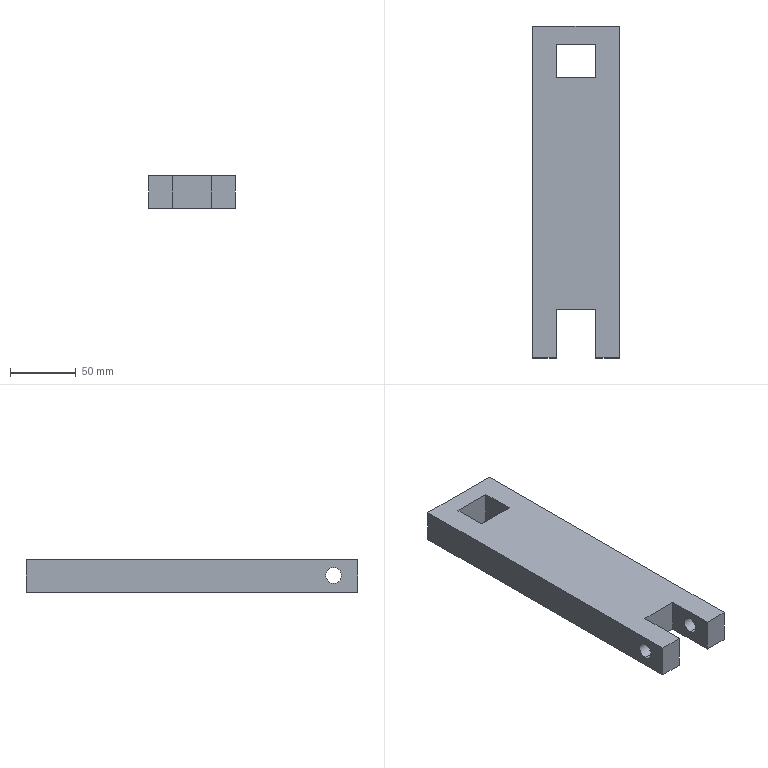Part | SolidWorks | features ICE 2, 3DProfileFeature 1, Extrusion 1, HoleWzd 1, MirrorPattern 1 | 1 solid | 18 faces | box 66 x 252 x 25 mm | volume 365157 mm3 | plane 14 | cylinder 4 | commonest cylinder face diameters 12 x4
STEP:
#1=CARTESIAN_POINT('',(-15.,-131.5,-5.548));
#2=VERTEX_POINT('',#1);
#3=CARTESIAN_POINT('',(-15.,-131.5,6.452));
#4=VERTEX_POINT('',#3);
#5=CARTESIAN_POINT('',(-15.,-131.5,0.4516));
#6=DIRECTION('',(-1.,0.,0.));
#7=DIRECTION('',(0.,0.,1.));
#8=AXIS2_PLACEMENT_3D('',#5,#6,#7);
#9=CIRCLE('',#8,6.);
#10=EDGE_CURVE('',#2,#4,#9,.T.);
#11=ORIENTED_EDGE('',*,*,#10,.F.);
#12=CARTESIAN_POINT('',(-33.,-131.5,-5.548));
#13=VERTEX_POINT('',#12);
#14=CARTESIAN_POINT('',(-33.,-131.5,-5.548));
#15=DIRECTION('',(-1.,0.,0.));
#16=VECTOR('',#15,1000.);
#17=LINE('',#14,#16);
#18=EDGE_CURVE('',#2,#13,#17,.T.);
#19=ORIENTED_EDGE('',*,*,#18,.T.);
#20=CARTESIAN_POINT('',(-33.,-131.5,6.452));
#21=VERTEX_POINT('',#20);
#22=CARTESIAN_POINT('',(-33.,-131.5,0.4516));
#23=DIRECTION('',(-1.,0.,0.));
#24=DIRECTION('',(0.,0.,1.));
#25=AXIS2_PLACEMENT_3D('',#22,#23,#24);
#26=CIRCLE('',#25,6.);
#27=EDGE_CURVE('',#13,#21,#26,.T.);
#28=ORIENTED_EDGE('',*,*,#27,.T.);
#29=CARTESIAN_POINT('',(-33.,-131.5,6.452));
#30=DIRECTION('',(-1.,0.,0.));
#31=VECTOR('',#30,1000.);
#32=LINE('',#29,#31);
#33=EDGE_CURVE('',#4,#21,#32,.T.);
#34=ORIENTED_EDGE('',*,*,#33,.F.);
#35=EDGE_LOOP('',(#11,#19,#28,#34));
#36=FACE_OUTER_BOUND('',#35,.T.);
#37=CARTESIAN_POINT('',(-33.,-131.5,0.4516));
#38=DIRECTION('',(-1.,0.,0.));
#39=DIRECTION('',(0.,0.,1.));
#40=AXIS2_PLACEMENT_3D('',#37,#38,#39);
#41=CYLINDRICAL_SURFACE('',#40,6.);
#42=ADVANCED_FACE('',(#36),#41,.F.);
#43=CARTESIAN_POINT('',(15.,-131.5,6.452));
#44=VERTEX_POINT('',#43);
#45=CARTESIAN_POINT('',(15.,-131.5,-5.548));
#46=VERTEX_POINT('',#45);
#47=CARTESIAN_POINT('',(15.,-131.5,0.4516));
#48=DIRECTION('',(1.,0.,0.));
#49=DIRECTION('',(0.,0.,-1.));
#50=AXIS2_PLACEMENT_3D('',#47,#48,#49);
#51=CIRCLE('',#50,6.);
#52=EDGE_CURVE('',#44,#46,#51,.T.);
#53=ORIENTED_EDGE('',*,*,#52,.F.);
#54=CARTESIAN_POINT('',(33.,-131.5,6.452));
#55=VERTEX_POINT('',#54);
#56=CARTESIAN_POINT('',(33.,-131.5,6.452));
#57=DIRECTION('',(1.,0.,0.));
#58=VECTOR('',#57,1000.);
#59=LINE('',#56,#58);
#60=EDGE_CURVE('',#44,#55,#59,.T.);
#61=ORIENTED_EDGE('',*,*,#60,.T.);
#62=CARTESIAN_POINT('',(33.,-131.5,-5.548));
#63=VERTEX_POINT('',#62);
#64=CARTESIAN_POINT('',(33.,-131.5,0.4516));
#65=DIRECTION('',(1.,0.,0.));
#66=DIRECTION('',(0.,0.,-1.));
#67=AXIS2_PLACEMENT_3D('',#64,#65,#66);
#68=CIRCLE('',#67,6.);
#69=EDGE_CURVE('',#55,#63,#68,.T.);
#70=ORIENTED_EDGE('',*,*,#69,.T.);
#71=CARTESIAN_POINT('',(33.,-131.5,-5.548));
#72=DIRECTION('',(1.,0.,0.));
#73=VECTOR('',#72,1000.);
#74=LINE('',#71,#73);
#75=EDGE_CURVE('',#46,#63,#74,.T.);
#76=ORIENTED_EDGE('',*,*,#75,.F.);
#77=EDGE_LOOP('',(#53,#61,#70,#76));
#78=FACE_OUTER_BOUND('',#77,.T.);
#79=CARTESIAN_POINT('',(33.,-131.5,0.4516));
#80=DIRECTION('',(1.,0.,0.));
#81=DIRECTION('',(0.,0.,-1.));
#82=AXIS2_PLACEMENT_3D('',#79,#80,#81);
#83=CYLINDRICAL_SURFACE('',#82,6.);
#84=ADVANCED_FACE('',(#78),#83,.F.);
#85=CARTESIAN_POINT('',(33.,-150.,-12.5));
#86=VERTEX_POINT('',#85);
#87=CARTESIAN_POINT('',(33.,102.,-12.5));
#88=VERTEX_POINT('',#87);
#89=CARTESIAN_POINT('',(33.,-150.,-12.5));
#90=DIRECTION('',(0.,1.,0.));
#91=VECTOR('',#90,1000.);
#92=LINE('',#89,#91);
#93=EDGE_CURVE('',#86,#88,#92,.T.);
#94=ORIENTED_EDGE('',*,*,#93,.T.);
#95=CARTESIAN_POINT('',(33.,102.,12.5));
#96=VERTEX_POINT('',#95);
#97=CARTESIAN_POINT('',(33.,102.,12.5));
#98=DIRECTION('',(0.,0.,-1.));
#99=VECTOR('',#98,1000.);
#100=LINE('',#97,#99);
#101=EDGE_CURVE('',#96,#88,#100,.T.);
#102=ORIENTED_EDGE('',*,*,#101,.F.);
#103=CARTESIAN_POINT('',(33.,-150.,12.5));
#104=VERTEX_POINT('',#103);
#105=CARTESIAN_POINT('',(33.,-150.,12.5));
#106=DIRECTION('',(0.,1.,0.));
#107=VECTOR('',#106,1000.);
#108=LINE('',#105,#107);
#109=EDGE_CURVE('',#104,#96,#108,.T.);
#110=ORIENTED_EDGE('',*,*,#109,.F.);
#111=CARTESIAN_POINT('',(33.,-150.,12.5));
#112=DIRECTION('',(0.,0.,-1.));
#113=VECTOR('',#112,1000.);
#114=LINE('',#111,#113);
#115=EDGE_CURVE('',#104,#86,#114,.T.);
#116=ORIENTED_EDGE('',*,*,#115,.T.);
#117=EDGE_LOOP('',(#94,#102,#110,#116));
#118=FACE_OUTER_BOUND('',#117,.T.);
#119=CARTESIAN_POINT('',(33.,-131.5,0.4516));
#120=DIRECTION('',(1.,0.,0.));
#121=DIRECTION('',(0.,0.,-1.));
#122=AXIS2_PLACEMENT_3D('',#119,#120,#121);
#123=CIRCLE('',#122,6.);
#124=EDGE_CURVE('',#63,#55,#123,.T.);
#125=ORIENTED_EDGE('',*,*,#124,.F.);
#126=ORIENTED_EDGE('',*,*,#69,.F.);
#127=EDGE_LOOP('',(#125,#126));
#128=FACE_BOUND('',#127,.T.);
#129=CARTESIAN_POINT('',(33.,-150.,12.5));
#130=DIRECTION('',(-1.,0.,0.));
#131=DIRECTION('',(0.,-1.,0.));
#132=AXIS2_PLACEMENT_3D('',#129,#130,#131);
#133=PLANE('',#132);
#134=ADVANCED_FACE('',(#118,#128),#133,.F.);
#135=CARTESIAN_POINT('',(-33.,-131.5,0.4516));
#136=DIRECTION('',(-1.,0.,0.));
#137=DIRECTION('',(0.,0.,1.));
#138=AXIS2_PLACEMENT_3D('',#135,#136,#137);
#139=CIRCLE('',#138,6.);
#140=EDGE_CURVE('',#21,#13,#139,.T.);
#141=ORIENTED_EDGE('',*,*,#140,.F.);
#142=ORIENTED_EDGE('',*,*,#27,.F.);
#143=EDGE_LOOP('',(#141,#142));
#144=FACE_BOUND('',#143,.T.);
#145=CARTESIAN_POINT('',(-33.,102.,-12.5));
#146=VERTEX_POINT('',#145);
#147=CARTESIAN_POINT('',(-33.,-150.,-12.5));
#148=VERTEX_POINT('',#147);
#149=CARTESIAN_POINT('',(-33.,-150.,-12.5));
#150=DIRECTION('',(0.,-1.,0.));
#151=VECTOR('',#150,1000.);
#152=LINE('',#149,#151);
#153=EDGE_CURVE('',#146,#148,#152,.T.);
#154=ORIENTED_EDGE('',*,*,#153,.T.);
#155=CARTESIAN_POINT('',(-33.,-150.,12.5));
#156=VERTEX_POINT('',#155);
#157=CARTESIAN_POINT('',(-33.,-150.,12.5));
#158=DIRECTION('',(0.,0.,-1.));
#159=VECTOR('',#158,1000.);
#160=LINE('',#157,#159);
#161=EDGE_CURVE('',#156,#148,#160,.T.);
#162=ORIENTED_EDGE('',*,*,#161,.F.);
#163=CARTESIAN_POINT('',(-33.,102.,12.5));
#164=VERTEX_POINT('',#163);
#165=CARTESIAN_POINT('',(-33.,-150.,12.5));
#166=DIRECTION('',(0.,-1.,0.));
#167=VECTOR('',#166,1000.);
#168=LINE('',#165,#167);
#169=EDGE_CURVE('',#164,#156,#168,.T.);
#170=ORIENTED_EDGE('',*,*,#169,.F.);
#171=CARTESIAN_POINT('',(-33.,102.,-12.5));
#172=DIRECTION('',(0.,0.,1.));
#173=VECTOR('',#172,1000.);
#174=LINE('',#171,#173);
#175=EDGE_CURVE('',#146,#164,#174,.T.);
#176=ORIENTED_EDGE('',*,*,#175,.F.);
#177=EDGE_LOOP('',(#154,#162,#170,#176));
#178=FACE_OUTER_BOUND('',#177,.T.);
#179=CARTESIAN_POINT('',(-33.,-150.,12.5));
#180=DIRECTION('',(1.,0.,0.));
#181=DIRECTION('',(0.,0.,-1.));
#182=AXIS2_PLACEMENT_3D('',#179,#180,#181);
#183=PLANE('',#182);
#184=ADVANCED_FACE('',(#144,#178),#183,.F.);
#185=CARTESIAN_POINT('',(-15.,-150.,-12.5));
#186=VERTEX_POINT('',#185);
#187=CARTESIAN_POINT('',(-33.,-150.,-12.5));
#188=DIRECTION('',(1.,0.,0.));
#189=VECTOR('',#188,1000.);
#190=LINE('',#187,#189);
#191=EDGE_CURVE('',#148,#186,#190,.T.);
#192=ORIENTED_EDGE('',*,*,#191,.T.);
#193=CARTESIAN_POINT('',(-15.,-150.,12.5));
#194=VERTEX_POINT('',#193);
#195=CARTESIAN_POINT('',(-15.,-150.,12.5));
#196=DIRECTION('',(0.,0.,-1.));
#197=VECTOR('',#196,1000.);
#198=LINE('',#195,#197);
#199=EDGE_CURVE('',#194,#186,#198,.T.);
#200=ORIENTED_EDGE('',*,*,#199,.F.);
#201=CARTESIAN_POINT('',(-33.,-150.,12.5));
#202=DIRECTION('',(1.,0.,0.));
#203=VECTOR('',#202,1000.);
#204=LINE('',#201,#203);
#205=EDGE_CURVE('',#156,#194,#204,.T.);
#206=ORIENTED_EDGE('',*,*,#205,.F.);
#207=ORIENTED_EDGE('',*,*,#161,.T.);
#208=EDGE_LOOP('',(#192,#200,#206,#207));
#209=FACE_OUTER_BOUND('',#208,.T.);
#210=CARTESIAN_POINT('',(-33.,-150.,12.5));
#211=DIRECTION('',(0.,1.,0.));
#212=DIRECTION('',(0.,0.,1.));
#213=AXIS2_PLACEMENT_3D('',#210,#211,#212);
#214=PLANE('',#213);
#215=ADVANCED_FACE('',(#209),#214,.F.);
#216=CARTESIAN_POINT('',(-15.,-131.5,0.4516));
#217=DIRECTION('',(-1.,0.,0.));
#218=DIRECTION('',(0.,0.,1.));
#219=AXIS2_PLACEMENT_3D('',#216,#217,#218);
#220=CIRCLE('',#219,6.);
#221=EDGE_CURVE('',#4,#2,#220,.T.);
#222=ORIENTED_EDGE('',*,*,#221,.T.);
#223=ORIENTED_EDGE('',*,*,#10,.T.);
#224=EDGE_LOOP('',(#222,#223));
#225=FACE_BOUND('',#224,.T.);
#226=CARTESIAN_POINT('',(-15.,-112.904,-12.5));
#227=VERTEX_POINT('',#226);
#228=CARTESIAN_POINT('',(-15.,-112.904,-12.5));
#229=DIRECTION('',(0.,1.,0.));
#230=VECTOR('',#229,1000.);
#231=LINE('',#228,#230);
#232=EDGE_CURVE('',#186,#227,#231,.T.);
#233=ORIENTED_EDGE('',*,*,#232,.T.);
#234=CARTESIAN_POINT('',(-15.,-112.904,12.5));
#235=VERTEX_POINT('',#234);
#236=CARTESIAN_POINT('',(-15.,-112.904,12.5));
#237=DIRECTION('',(0.,0.,-1.));
#238=VECTOR('',#237,1000.);
#239=LINE('',#236,#238);
#240=EDGE_CURVE('',#235,#227,#239,.T.);
#241=ORIENTED_EDGE('',*,*,#240,.F.);
#242=CARTESIAN_POINT('',(-15.,-112.904,12.5));
#243=DIRECTION('',(0.,1.,0.));
#244=VECTOR('',#243,1000.);
#245=LINE('',#242,#244);
#246=EDGE_CURVE('',#194,#235,#245,.T.);
#247=ORIENTED_EDGE('',*,*,#246,.F.);
#248=ORIENTED_EDGE('',*,*,#199,.T.);
#249=EDGE_LOOP('',(#233,#241,#247,#248));
#250=FACE_OUTER_BOUND('',#249,.T.);
#251=CARTESIAN_POINT('',(-15.,-112.904,12.5));
#252=DIRECTION('',(-1.,0.,0.));
#253=DIRECTION('',(0.,0.,1.));
#254=AXIS2_PLACEMENT_3D('',#251,#252,#253);
#255=PLANE('',#254);
#256=ADVANCED_FACE('',(#225,#250),#255,.F.);
#257=CARTESIAN_POINT('',(15.,-112.904,-12.5));
#258=VERTEX_POINT('',#257);
#259=CARTESIAN_POINT('',(0.,-112.904,-12.5));
#260=DIRECTION('',(1.,0.,0.));
#261=VECTOR('',#260,1000.);
#262=LINE('',#259,#261);
#263=EDGE_CURVE('',#227,#258,#262,.T.);
#264=ORIENTED_EDGE('',*,*,#263,.T.);
#265=CARTESIAN_POINT('',(15.,-112.904,12.5));
#266=VERTEX_POINT('',#265);
#267=CARTESIAN_POINT('',(15.,-112.904,12.5));
#268=DIRECTION('',(0.,0.,-1.));
#269=VECTOR('',#268,1000.);
#270=LINE('',#267,#269);
#271=EDGE_CURVE('',#266,#258,#270,.T.);
#272=ORIENTED_EDGE('',*,*,#271,.F.);
#273=CARTESIAN_POINT('',(0.,-112.904,12.5));
#274=DIRECTION('',(1.,0.,0.));
#275=VECTOR('',#274,1000.);
#276=LINE('',#273,#275);
#277=EDGE_CURVE('',#235,#266,#276,.T.);
#278=ORIENTED_EDGE('',*,*,#277,.F.);
#279=ORIENTED_EDGE('',*,*,#240,.T.);
#280=EDGE_LOOP('',(#264,#272,#278,#279));
#281=FACE_OUTER_BOUND('',#280,.T.);
#282=CARTESIAN_POINT('',(0.,-112.904,12.5));
#283=DIRECTION('',(0.,1.,0.));
#284=DIRECTION('',(0.,0.,1.));
#285=AXIS2_PLACEMENT_3D('',#282,#283,#284);
#286=PLANE('',#285);
#287=ADVANCED_FACE('',(#281),#286,.F.);
#288=CARTESIAN_POINT('',(15.,-131.5,0.4516));
#289=DIRECTION('',(1.,0.,0.));
#290=DIRECTION('',(0.,0.,-1.));
#291=AXIS2_PLACEMENT_3D('',#288,#289,#290);
#292=CIRCLE('',#291,6.);
#293=EDGE_CURVE('',#46,#44,#292,.T.);
#294=ORIENTED_EDGE('',*,*,#293,.T.);
#295=ORIENTED_EDGE('',*,*,#52,.T.);
#296=EDGE_LOOP('',(#294,#295));
#297=FACE_BOUND('',#296,.T.);
#298=CARTESIAN_POINT('',(15.,-150.,-12.5));
#299=VERTEX_POINT('',#298);
#300=CARTESIAN_POINT('',(15.,-112.904,-12.5));
#301=DIRECTION('',(0.,-1.,0.));
#302=VECTOR('',#301,1000.);
#303=LINE('',#300,#302);
#304=EDGE_CURVE('',#258,#299,#303,.T.);
#305=ORIENTED_EDGE('',*,*,#304,.T.);
#306=CARTESIAN_POINT('',(15.,-150.,12.5));
#307=VERTEX_POINT('',#306);
#308=CARTESIAN_POINT('',(15.,-150.,12.5));
#309=DIRECTION('',(0.,0.,-1.));
#310=VECTOR('',#309,1000.);
#311=LINE('',#308,#310);
#312=EDGE_CURVE('',#307,#299,#311,.T.);
#313=ORIENTED_EDGE('',*,*,#312,.F.);
#314=CARTESIAN_POINT('',(15.,-112.904,12.5));
#315=DIRECTION('',(0.,-1.,0.));
#316=VECTOR('',#315,1000.);
#317=LINE('',#314,#316);
#318=EDGE_CURVE('',#266,#307,#317,.T.);
#319=ORIENTED_EDGE('',*,*,#318,.F.);
#320=ORIENTED_EDGE('',*,*,#271,.T.);
#321=EDGE_LOOP('',(#305,#313,#319,#320));
#322=FACE_OUTER_BOUND('',#321,.T.);
#323=CARTESIAN_POINT('',(15.,-112.904,12.5));
#324=DIRECTION('',(1.,0.,0.));
#325=DIRECTION('',(0.,0.,-1.));
#326=AXIS2_PLACEMENT_3D('',#323,#324,#325);
#327=PLANE('',#326);
#328=ADVANCED_FACE('',(#297,#322),#327,.F.);
#329=CARTESIAN_POINT('',(15.,-150.,-12.5));
#330=DIRECTION('',(1.,0.,0.));
#331=VECTOR('',#330,1000.);
#332=LINE('',#329,#331);
#333=EDGE_CURVE('',#299,#86,#332,.T.);
#334=ORIENTED_EDGE('',*,*,#333,.T.);
#335=ORIENTED_EDGE('',*,*,#115,.F.);
#336=CARTESIAN_POINT('',(15.,-150.,12.5));
#337=DIRECTION('',(1.,0.,0.));
#338=VECTOR('',#337,1000.);
#339=LINE('',#336,#338);
#340=EDGE_CURVE('',#307,#104,#339,.T.);
#341=ORIENTED_EDGE('',*,*,#340,.F.);
#342=ORIENTED_EDGE('',*,*,#312,.T.);
#343=EDGE_LOOP('',(#334,#335,#341,#342));
#344=FACE_OUTER_BOUND('',#343,.T.);
#345=CARTESIAN_POINT('',(15.,-150.,12.5));
#346=DIRECTION('',(0.,1.,0.));
#347=DIRECTION('',(0.,0.,1.));
#348=AXIS2_PLACEMENT_3D('',#345,#346,#347);
#349=PLANE('',#348);
#350=ADVANCED_FACE('',(#344),#349,.F.);
#351=CARTESIAN_POINT('',(15.,87.705,12.5));
#352=VERTEX_POINT('',#351);
#353=CARTESIAN_POINT('',(15.,62.705,12.5));
#354=VERTEX_POINT('',#353);
#355=CARTESIAN_POINT('',(15.,62.705,12.5));
#356=DIRECTION('',(0.,-1.,0.));
#357=VECTOR('',#356,1000.);
#358=LINE('',#355,#357);
#359=EDGE_CURVE('',#352,#354,#358,.T.);
#360=ORIENTED_EDGE('',*,*,#359,.T.);
#361=CARTESIAN_POINT('',(-15.,62.705,12.5));
#362=VERTEX_POINT('',#361);
#363=CARTESIAN_POINT('',(15.,62.705,12.5));
#364=DIRECTION('',(-1.,0.,0.));
#365=VECTOR('',#364,1000.);
#366=LINE('',#363,#365);
#367=EDGE_CURVE('',#354,#362,#366,.T.);
#368=ORIENTED_EDGE('',*,*,#367,.T.);
#369=CARTESIAN_POINT('',(-15.,87.705,12.5));
#370=VERTEX_POINT('',#369);
#371=CARTESIAN_POINT('',(-15.,62.705,12.5));
#372=DIRECTION('',(0.,1.,0.));
#373=VECTOR('',#372,1000.);
#374=LINE('',#371,#373);
#375=EDGE_CURVE('',#362,#370,#374,.T.);
#376=ORIENTED_EDGE('',*,*,#375,.T.);
#377=CARTESIAN_POINT('',(15.,87.705,12.5));
#378=DIRECTION('',(1.,0.,0.));
#379=VECTOR('',#378,1000.);
#380=LINE('',#377,#379);
#381=EDGE_CURVE('',#370,#352,#380,.T.);
#382=ORIENTED_EDGE('',*,*,#381,.T.);
#383=EDGE_LOOP('',(#360,#368,#376,#382));
#384=FACE_BOUND('',#383,.T.);
#385=ORIENTED_EDGE('',*,*,#109,.T.);
#386=CARTESIAN_POINT('',(-33.,102.,12.5));
#387=DIRECTION('',(1.,0.,0.));
#388=VECTOR('',#387,1000.);
#389=LINE('',#386,#388);
#390=EDGE_CURVE('',#164,#96,#389,.T.);
#391=ORIENTED_EDGE('',*,*,#390,.F.);
#392=ORIENTED_EDGE('',*,*,#169,.T.);
#393=ORIENTED_EDGE('',*,*,#205,.T.);
#394=ORIENTED_EDGE('',*,*,#246,.T.);
#395=ORIENTED_EDGE('',*,*,#277,.T.);
#396=ORIENTED_EDGE('',*,*,#318,.T.);
#397=ORIENTED_EDGE('',*,*,#340,.T.);
#398=EDGE_LOOP('',(#385,#391,#392,#393,#394,#395,#396,#397));
#399=FACE_OUTER_BOUND('',#398,.T.);
#400=CARTESIAN_POINT('',(0.,0.,12.5));
#401=DIRECTION('',(0.,0.,1.));
#402=DIRECTION('',(1.,0.,0.));
#403=AXIS2_PLACEMENT_3D('',#400,#401,#402);
#404=PLANE('',#403);
#405=ADVANCED_FACE('',(#384,#399),#404,.T.);
#406=CARTESIAN_POINT('',(15.,62.705,-12.5));
#407=VERTEX_POINT('',#406);
#408=CARTESIAN_POINT('',(-15.,62.705,-12.5));
#409=VERTEX_POINT('',#408);
#410=CARTESIAN_POINT('',(15.,62.705,-12.5));
#411=DIRECTION('',(-1.,0.,0.));
#412=VECTOR('',#411,1000.);
#413=LINE('',#410,#412);
#414=EDGE_CURVE('',#407,#409,#413,.T.);
#415=ORIENTED_EDGE('',*,*,#414,.F.);
#416=CARTESIAN_POINT('',(15.,87.705,-12.5));
#417=VERTEX_POINT('',#416);
#418=CARTESIAN_POINT('',(15.,62.705,-12.5));
#419=DIRECTION('',(0.,-1.,0.));
#420=VECTOR('',#419,1000.);
#421=LINE('',#418,#420);
#422=EDGE_CURVE('',#417,#407,#421,.T.);
#423=ORIENTED_EDGE('',*,*,#422,.F.);
#424=CARTESIAN_POINT('',(-15.,87.705,-12.5));
#425=VERTEX_POINT('',#424);
#426=CARTESIAN_POINT('',(15.,87.705,-12.5));
#427=DIRECTION('',(1.,0.,0.));
#428=VECTOR('',#427,1000.);
#429=LINE('',#426,#428);
#430=EDGE_CURVE('',#425,#417,#429,.T.);
#431=ORIENTED_EDGE('',*,*,#430,.F.);
#432=CARTESIAN_POINT('',(-15.,62.705,-12.5));
#433=DIRECTION('',(0.,1.,0.));
#434=VECTOR('',#433,1000.);
#435=LINE('',#432,#434);
#436=EDGE_CURVE('',#409,#425,#435,.T.);
#437=ORIENTED_EDGE('',*,*,#436,.F.);
#438=EDGE_LOOP('',(#415,#423,#431,#437));
#439=FACE_BOUND('',#438,.T.);
#440=ORIENTED_EDGE('',*,*,#153,.F.);
#441=CARTESIAN_POINT('',(33.,102.,-12.5));
#442=DIRECTION('',(-1.,0.,0.));
#443=VECTOR('',#442,1000.);
#444=LINE('',#441,#443);
#445=EDGE_CURVE('',#88,#146,#444,.T.);
#446=ORIENTED_EDGE('',*,*,#445,.F.);
#447=ORIENTED_EDGE('',*,*,#93,.F.);
#448=ORIENTED_EDGE('',*,*,#333,.F.);
#449=ORIENTED_EDGE('',*,*,#304,.F.);
#450=ORIENTED_EDGE('',*,*,#263,.F.);
#451=ORIENTED_EDGE('',*,*,#232,.F.);
#452=ORIENTED_EDGE('',*,*,#191,.F.);
#453=EDGE_LOOP('',(#440,#446,#447,#448,#449,#450,#451,#452));
#454=FACE_OUTER_BOUND('',#453,.T.);
#455=CARTESIAN_POINT('',(0.,0.,-12.5));
#456=DIRECTION('',(0.,0.,1.));
#457=DIRECTION('',(1.,0.,0.));
#458=AXIS2_PLACEMENT_3D('',#455,#456,#457);
#459=PLANE('',#458);
#460=ADVANCED_FACE('',(#439,#454),#459,.F.);
#461=ORIENTED_EDGE('',*,*,#60,.F.);
#462=ORIENTED_EDGE('',*,*,#293,.F.);
#463=ORIENTED_EDGE('',*,*,#75,.T.);
#464=ORIENTED_EDGE('',*,*,#124,.T.);
#465=EDGE_LOOP('',(#461,#462,#463,#464));
#466=FACE_OUTER_BOUND('',#465,.T.);
#467=CARTESIAN_POINT('',(33.,-131.5,0.4516));
#468=DIRECTION('',(1.,0.,0.));
#469=DIRECTION('',(0.,0.,-1.));
#470=AXIS2_PLACEMENT_3D('',#467,#468,#469);
#471=CYLINDRICAL_SURFACE('',#470,6.);
#472=ADVANCED_FACE('',(#466),#471,.F.);
#473=ORIENTED_EDGE('',*,*,#18,.F.);
#474=ORIENTED_EDGE('',*,*,#221,.F.);
#475=ORIENTED_EDGE('',*,*,#33,.T.);
#476=ORIENTED_EDGE('',*,*,#140,.T.);
#477=EDGE_LOOP('',(#473,#474,#475,#476));
#478=FACE_OUTER_BOUND('',#477,.T.);
#479=CARTESIAN_POINT('',(-33.,-131.5,0.4516));
#480=DIRECTION('',(-1.,0.,0.));
#481=DIRECTION('',(0.,0.,1.));
#482=AXIS2_PLACEMENT_3D('',#479,#480,#481);
#483=CYLINDRICAL_SURFACE('',#482,6.);
#484=ADVANCED_FACE('',(#478),#483,.F.);
#485=ORIENTED_EDGE('',*,*,#101,.T.);
#486=ORIENTED_EDGE('',*,*,#445,.T.);
#487=ORIENTED_EDGE('',*,*,#175,.T.);
#488=ORIENTED_EDGE('',*,*,#390,.T.);
#489=EDGE_LOOP('',(#485,#486,#487,#488));
#490=FACE_OUTER_BOUND('',#489,.T.);
#491=CARTESIAN_POINT('',(0.,102.,0.));
#492=DIRECTION('',(0.,1.,0.));
#493=DIRECTION('',(0.,0.,1.));
#494=AXIS2_PLACEMENT_3D('',#491,#492,#493);
#495=PLANE('',#494);
#496=ADVANCED_FACE('',(#490),#495,.T.);
#497=ORIENTED_EDGE('',*,*,#422,.T.);
#498=CARTESIAN_POINT('',(15.,62.705,12.5));
#499=DIRECTION('',(0.,0.,-1.));
#500=VECTOR('',#499,1000.);
#501=LINE('',#498,#500);
#502=EDGE_CURVE('',#354,#407,#501,.T.);
#503=ORIENTED_EDGE('',*,*,#502,.F.);
#504=ORIENTED_EDGE('',*,*,#359,.F.);
#505=CARTESIAN_POINT('',(15.,87.705,12.5));
#506=DIRECTION('',(0.,0.,-1.));
#507=VECTOR('',#506,1000.);
#508=LINE('',#505,#507);
#509=EDGE_CURVE('',#352,#417,#508,.T.);
#510=ORIENTED_EDGE('',*,*,#509,.T.);
#511=EDGE_LOOP('',(#497,#503,#504,#510));
#512=FACE_OUTER_BOUND('',#511,.T.);
#513=CARTESIAN_POINT('',(15.,62.705,12.5));
#514=DIRECTION('',(1.,0.,0.));
#515=DIRECTION('',(0.,0.,-1.));
#516=AXIS2_PLACEMENT_3D('',#513,#514,#515);
#517=PLANE('',#516);
#518=ADVANCED_FACE('',(#512),#517,.F.);
#519=ORIENTED_EDGE('',*,*,#430,.T.);
#520=ORIENTED_EDGE('',*,*,#509,.F.);
#521=ORIENTED_EDGE('',*,*,#381,.F.);
#522=CARTESIAN_POINT('',(-15.,87.705,12.5));
#523=DIRECTION('',(0.,0.,-1.));
#524=VECTOR('',#523,1000.);
#525=LINE('',#522,#524);
#526=EDGE_CURVE('',#370,#425,#525,.T.);
#527=ORIENTED_EDGE('',*,*,#526,.T.);
#528=EDGE_LOOP('',(#519,#520,#521,#527));
#529=FACE_OUTER_BOUND('',#528,.T.);
#530=CARTESIAN_POINT('',(15.,87.705,12.5));
#531=DIRECTION('',(0.,1.,0.));
#532=DIRECTION('',(0.,0.,1.));
#533=AXIS2_PLACEMENT_3D('',#530,#531,#532);
#534=PLANE('',#533);
#535=ADVANCED_FACE('',(#529),#534,.F.);
#536=ORIENTED_EDGE('',*,*,#436,.T.);
#537=ORIENTED_EDGE('',*,*,#526,.F.);
#538=ORIENTED_EDGE('',*,*,#375,.F.);
#539=CARTESIAN_POINT('',(-15.,62.705,12.5));
#540=DIRECTION('',(0.,0.,-1.));
#541=VECTOR('',#540,1000.);
#542=LINE('',#539,#541);
#543=EDGE_CURVE('',#362,#409,#542,.T.);
#544=ORIENTED_EDGE('',*,*,#543,.T.);
#545=EDGE_LOOP('',(#536,#537,#538,#544));
#546=FACE_OUTER_BOUND('',#545,.T.);
#547=CARTESIAN_POINT('',(-15.,62.705,12.5));
#548=DIRECTION('',(-1.,0.,0.));
#549=DIRECTION('',(0.,0.,1.));
#550=AXIS2_PLACEMENT_3D('',#547,#548,#549);
#551=PLANE('',#550);
#552=ADVANCED_FACE('',(#546),#551,.F.);
#553=ORIENTED_EDGE('',*,*,#414,.T.);
#554=ORIENTED_EDGE('',*,*,#543,.F.);
#555=ORIENTED_EDGE('',*,*,#367,.F.);
#556=ORIENTED_EDGE('',*,*,#502,.T.);
#557=EDGE_LOOP('',(#553,#554,#555,#556));
#558=FACE_OUTER_BOUND('',#557,.T.);
#559=CARTESIAN_POINT('',(15.,62.705,12.5));
#560=DIRECTION('',(0.,-1.,0.));
#561=DIRECTION('',(0.,0.,-1.));
#562=AXIS2_PLACEMENT_3D('',#559,#560,#561);
#563=PLANE('',#562);
#564=ADVANCED_FACE('',(#558),#563,.F.);
#565=CLOSED_SHELL('',(#42,#84,#134,#184,#215,#256,#287,#328,#350,#405,#460,#472,#484,#496,#518,#535,#552,#564));
#566=MANIFOLD_SOLID_BREP('',#565);
#567=CARTESIAN_POINT('',(0.,0.,0.));
#568=DIRECTION('',(0.,0.,1.));
#569=DIRECTION('',(1.,0.,0.));
#570=AXIS2_PLACEMENT_3D('',#567,#568,#569);
#571=(LENGTH_UNIT()NAMED_UNIT(*)SI_UNIT(.MILLI.,.METRE.));
#572=UNCERTAINTY_MEASURE_WITH_UNIT(LENGTH_MEASURE(0.00001),#571,'','');
#573=(NAMED_UNIT(*)PLANE_ANGLE_UNIT()SI_UNIT($,.RADIAN.));
#574=(NAMED_UNIT(*)SI_UNIT($,.STERADIAN.)SOLID_ANGLE_UNIT());
#575=(GEOMETRIC_REPRESENTATION_CONTEXT(3)GLOBAL_UNCERTAINTY_ASSIGNED_CONTEXT((#572))GLOBAL_UNIT_ASSIGNED_CONTEXT((#571,#573,#574))REPRESENTATION_CONTEXT('',''));
#576=ADVANCED_BREP_SHAPE_REPRESENTATION('',(#566,#570),#575);